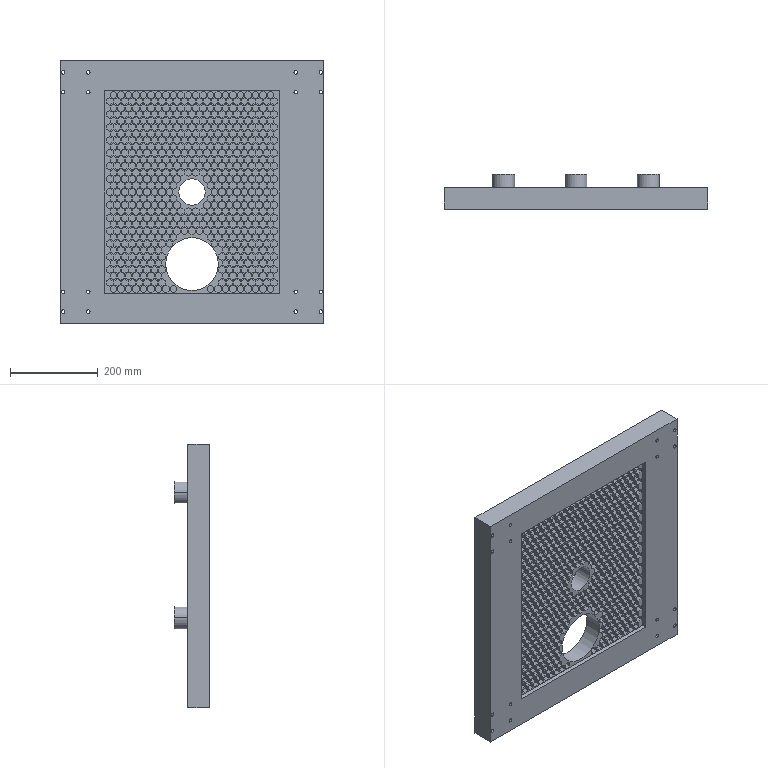Part | STEP file | 2026.6.15-Main Assembly图.sldasm-Part-75 | 1 solid | 4396 faces | volume 14522910 mm3 | plane 4354 | cylinder 42 | commonest cylinder face diameters 8 x32 50 x6 60 x2 120 x2